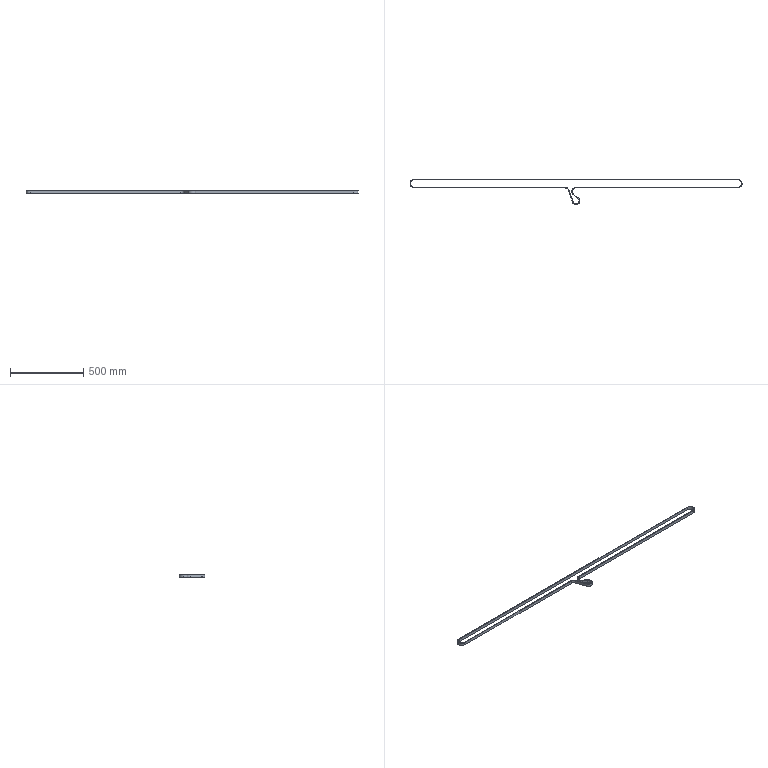Part | STEP file | Guide wheel mechanism revised.sldasm-Part-73 | 1 solid | 26 faces | box 2259 x 173.965 x 20 mm | volume 434312 mm3 | cylinder 14 | plane 12 | commonest cylinder face diameters 50 x6 59 x6 41.93 x1 51.93 x1
STEP:
#1=CARTESIAN_POINT('',(1081.857,-77.761,10.));
#2=VERTEX_POINT('',#1);
#3=CARTESIAN_POINT('',(1070.5,-54.5,10.));
#4=VERTEX_POINT('',#3);
#5=CARTESIAN_POINT('',(1100.,-54.5,10.));
#6=DIRECTION('',(0.,0.,-1.));
#7=DIRECTION('',(-1.,0.,0.));
#8=AXIS2_PLACEMENT_3D('',#5,#6,#7);
#9=CIRCLE('',#8,29.5);
#10=EDGE_CURVE('',#2,#4,#9,.T.);
#11=ORIENTED_EDGE('',*,*,#10,.T.);
#12=CARTESIAN_POINT('',(1070.5,-54.5,-10.));
#13=VERTEX_POINT('',#12);
#14=CARTESIAN_POINT('',(1070.5,-54.5,10.));
#15=DIRECTION('',(0.,0.,-1.));
#16=VECTOR('',#15,1000.);
#17=LINE('',#14,#16);
#18=EDGE_CURVE('',#4,#13,#17,.T.);
#19=ORIENTED_EDGE('',*,*,#18,.T.);
#20=CARTESIAN_POINT('',(1081.857,-77.761,-10.));
#21=VERTEX_POINT('',#20);
#22=CARTESIAN_POINT('',(1100.,-54.5,-10.));
#23=DIRECTION('',(0.,0.,-1.));
#24=DIRECTION('',(-1.,0.,0.));
#25=AXIS2_PLACEMENT_3D('',#22,#23,#24);
#26=CIRCLE('',#25,29.5);
#27=EDGE_CURVE('',#21,#13,#26,.T.);
#28=ORIENTED_EDGE('',*,*,#27,.F.);
#29=CARTESIAN_POINT('',(1081.857,-77.761,10.));
#30=DIRECTION('',(0.,0.,-1.));
#31=VECTOR('',#30,1000.);
#32=LINE('',#29,#31);
#33=EDGE_CURVE('',#2,#21,#32,.T.);
#34=ORIENTED_EDGE('',*,*,#33,.F.);
#35=EDGE_LOOP('',(#11,#19,#28,#34));
#36=FACE_OUTER_BOUND('',#35,.T.);
#37=CARTESIAN_POINT('',(1100.,-54.5,10.));
#38=DIRECTION('',(0.,0.,-1.));
#39=DIRECTION('',(-1.,0.,0.));
#40=AXIS2_PLACEMENT_3D('',#37,#38,#39);
#41=CYLINDRICAL_SURFACE('',#40,29.5);
#42=ADVANCED_FACE('',(#36),#41,.T.);
#43=CARTESIAN_POINT('',(0.,25.,10.));
#44=VERTEX_POINT('',#43);
#45=CARTESIAN_POINT('',(-25.,0.,10.));
#46=VERTEX_POINT('',#45);
#47=CARTESIAN_POINT('',(0.,0.,10.));
#48=DIRECTION('',(0.,0.,1.));
#49=DIRECTION('',(1.,0.,0.));
#50=AXIS2_PLACEMENT_3D('',#47,#48,#49);
#51=CIRCLE('',#50,25.);
#52=EDGE_CURVE('',#44,#46,#51,.T.);
#53=ORIENTED_EDGE('',*,*,#52,.T.);
#54=CARTESIAN_POINT('',(-25.,0.,-10.));
#55=VERTEX_POINT('',#54);
#56=CARTESIAN_POINT('',(-25.,0.,10.));
#57=DIRECTION('',(0.,0.,-1.));
#58=VECTOR('',#57,1000.);
#59=LINE('',#56,#58);
#60=EDGE_CURVE('',#46,#55,#59,.T.);
#61=ORIENTED_EDGE('',*,*,#60,.T.);
#62=CARTESIAN_POINT('',(0.,25.,-10.));
#63=VERTEX_POINT('',#62);
#64=CARTESIAN_POINT('',(0.,0.,-10.));
#65=DIRECTION('',(0.,0.,1.));
#66=DIRECTION('',(1.,0.,0.));
#67=AXIS2_PLACEMENT_3D('',#64,#65,#66);
#68=CIRCLE('',#67,25.);
#69=EDGE_CURVE('',#63,#55,#68,.T.);
#70=ORIENTED_EDGE('',*,*,#69,.F.);
#71=CARTESIAN_POINT('',(0.,25.,10.));
#72=DIRECTION('',(0.,0.,-1.));
#73=VECTOR('',#72,1000.);
#74=LINE('',#71,#73);
#75=EDGE_CURVE('',#44,#63,#74,.T.);
#76=ORIENTED_EDGE('',*,*,#75,.F.);
#77=EDGE_LOOP('',(#53,#61,#70,#76));
#78=FACE_OUTER_BOUND('',#77,.T.);
#79=CARTESIAN_POINT('',(0.,0.,10.));
#80=DIRECTION('',(0.,0.,-1.));
#81=DIRECTION('',(-1.,0.,0.));
#82=AXIS2_PLACEMENT_3D('',#79,#80,#81);
#83=CYLINDRICAL_SURFACE('',#82,25.);
#84=ADVANCED_FACE('',(#78),#83,.F.);
#85=CARTESIAN_POINT('',(1075.,-54.5,10.));
#86=VERTEX_POINT('',#85);
#87=CARTESIAN_POINT('',(1100.,-29.5,10.));
#88=VERTEX_POINT('',#87);
#89=CARTESIAN_POINT('',(1100.,-54.5,10.));
#90=DIRECTION('',(0.,0.,-1.));
#91=DIRECTION('',(-1.,0.,0.));
#92=AXIS2_PLACEMENT_3D('',#89,#90,#91);
#93=CIRCLE('',#92,25.);
#94=EDGE_CURVE('',#86,#88,#93,.T.);
#95=ORIENTED_EDGE('',*,*,#94,.F.);
#96=CARTESIAN_POINT('',(1075.,-54.5,-10.));
#97=VERTEX_POINT('',#96);
#98=CARTESIAN_POINT('',(1075.,-54.5,10.));
#99=DIRECTION('',(0.,0.,-1.));
#100=VECTOR('',#99,1000.);
#101=LINE('',#98,#100);
#102=EDGE_CURVE('',#86,#97,#101,.T.);
#103=ORIENTED_EDGE('',*,*,#102,.T.);
#104=CARTESIAN_POINT('',(1100.,-29.5,-10.));
#105=VERTEX_POINT('',#104);
#106=CARTESIAN_POINT('',(1100.,-54.5,-10.));
#107=DIRECTION('',(0.,0.,-1.));
#108=DIRECTION('',(-1.,0.,0.));
#109=AXIS2_PLACEMENT_3D('',#106,#107,#108);
#110=CIRCLE('',#109,25.);
#111=EDGE_CURVE('',#97,#105,#110,.T.);
#112=ORIENTED_EDGE('',*,*,#111,.T.);
#113=CARTESIAN_POINT('',(1100.,-29.5,10.));
#114=DIRECTION('',(0.,0.,-1.));
#115=VECTOR('',#114,1000.);
#116=LINE('',#113,#115);
#117=EDGE_CURVE('',#88,#105,#116,.T.);
#118=ORIENTED_EDGE('',*,*,#117,.F.);
#119=EDGE_LOOP('',(#95,#103,#112,#118));
#120=FACE_OUTER_BOUND('',#119,.T.);
#121=CARTESIAN_POINT('',(1100.,-54.5,10.));
#122=DIRECTION('',(0.,0.,-1.));
#123=DIRECTION('',(-1.,0.,0.));
#124=AXIS2_PLACEMENT_3D('',#121,#122,#123);
#125=CYLINDRICAL_SURFACE('',#124,25.);
#126=ADVANCED_FACE('',(#120),#125,.F.);
#127=CARTESIAN_POINT('',(-29.5,0.,10.));
#128=VERTEX_POINT('',#127);
#129=CARTESIAN_POINT('',(0.,-29.5,10.));
#130=VERTEX_POINT('',#129);
#131=CARTESIAN_POINT('',(0.,0.,10.));
#132=DIRECTION('',(0.,0.,1.));
#133=DIRECTION('',(1.,0.,0.));
#134=AXIS2_PLACEMENT_3D('',#131,#132,#133);
#135=CIRCLE('',#134,29.5);
#136=EDGE_CURVE('',#128,#130,#135,.T.);
#137=ORIENTED_EDGE('',*,*,#136,.F.);
#138=CARTESIAN_POINT('',(-29.5,0.,-10.));
#139=VERTEX_POINT('',#138);
#140=CARTESIAN_POINT('',(-29.5,0.,10.));
#141=DIRECTION('',(0.,0.,-1.));
#142=VECTOR('',#141,1000.);
#143=LINE('',#140,#142);
#144=EDGE_CURVE('',#128,#139,#143,.T.);
#145=ORIENTED_EDGE('',*,*,#144,.T.);
#146=CARTESIAN_POINT('',(0.,-29.5,-10.));
#147=VERTEX_POINT('',#146);
#148=CARTESIAN_POINT('',(0.,0.,-10.));
#149=DIRECTION('',(0.,0.,1.));
#150=DIRECTION('',(1.,0.,0.));
#151=AXIS2_PLACEMENT_3D('',#148,#149,#150);
#152=CIRCLE('',#151,29.5);
#153=EDGE_CURVE('',#139,#147,#152,.T.);
#154=ORIENTED_EDGE('',*,*,#153,.T.);
#155=CARTESIAN_POINT('',(0.,-29.5,10.));
#156=DIRECTION('',(0.,0.,-1.));
#157=VECTOR('',#156,1000.);
#158=LINE('',#155,#157);
#159=EDGE_CURVE('',#130,#147,#158,.T.);
#160=ORIENTED_EDGE('',*,*,#159,.F.);
#161=EDGE_LOOP('',(#137,#145,#154,#160));
#162=FACE_OUTER_BOUND('',#161,.T.);
#163=CARTESIAN_POINT('',(0.,0.,10.));
#164=DIRECTION('',(0.,0.,-1.));
#165=DIRECTION('',(-1.,0.,0.));
#166=AXIS2_PLACEMENT_3D('',#163,#164,#165);
#167=CYLINDRICAL_SURFACE('',#166,29.5);
#168=ADVANCED_FACE('',(#162),#167,.T.);
#169=CARTESIAN_POINT('',(0.,29.5,10.));
#170=VERTEX_POINT('',#169);
#171=CARTESIAN_POINT('',(0.,0.,10.));
#172=DIRECTION('',(0.,0.,1.));
#173=DIRECTION('',(1.,0.,0.));
#174=AXIS2_PLACEMENT_3D('',#171,#172,#173);
#175=CIRCLE('',#174,29.5);
#176=EDGE_CURVE('',#170,#128,#175,.T.);
#177=ORIENTED_EDGE('',*,*,#176,.T.);
#178=ORIENTED_EDGE('',*,*,#136,.T.);
#179=CARTESIAN_POINT('',(1025.,-29.5,10.));
#180=VERTEX_POINT('',#179);
#181=CARTESIAN_POINT('',(0.,-29.5,10.));
#182=DIRECTION('',(1.,0.,0.));
#183=VECTOR('',#182,1000.);
#184=LINE('',#181,#183);
#185=EDGE_CURVE('',#130,#180,#184,.T.);
#186=ORIENTED_EDGE('',*,*,#185,.T.);
#187=CARTESIAN_POINT('',(1048.722,-46.609,10.));
#188=VERTEX_POINT('',#187);
#189=CARTESIAN_POINT('',(1025.,-54.5,10.));
#190=DIRECTION('',(0.,0.,-1.));
#191=DIRECTION('',(-1.,0.,0.));
#192=AXIS2_PLACEMENT_3D('',#189,#190,#191);
#193=CIRCLE('',#192,25.);
#194=EDGE_CURVE('',#180,#188,#193,.T.);
#195=ORIENTED_EDGE('',*,*,#194,.T.);
#196=CARTESIAN_POINT('',(1075.362,-126.696,10.));
#197=VERTEX_POINT('',#196);
#198=CARTESIAN_POINT('',(1048.722,-46.609,10.));
#199=DIRECTION('',(0.3156,-0.9489,0.));
#200=VECTOR('',#199,1000.);
#201=LINE('',#198,#200);
#202=EDGE_CURVE('',#188,#197,#201,.T.);
#203=ORIENTED_EDGE('',*,*,#202,.T.);
#204=CARTESIAN_POINT('',(1115.705,-97.823,10.));
#205=VERTEX_POINT('',#204);
#206=CARTESIAN_POINT('',(1100.,-118.5,10.));
#207=DIRECTION('',(0.,0.,1.));
#208=DIRECTION('',(1.,0.,0.));
#209=AXIS2_PLACEMENT_3D('',#206,#207,#208);
#210=CIRCLE('',#209,25.965);
#211=EDGE_CURVE('',#197,#205,#210,.T.);
#212=ORIENTED_EDGE('',*,*,#211,.T.);
#213=CARTESIAN_POINT('',(1084.878,-74.408,10.));
#214=VERTEX_POINT('',#213);
#215=CARTESIAN_POINT('',(1115.705,-97.823,10.));
#216=DIRECTION('',(-0.7963,0.6049,0.));
#217=VECTOR('',#216,1000.);
#218=LINE('',#215,#217);
#219=EDGE_CURVE('',#205,#214,#218,.T.);
#220=ORIENTED_EDGE('',*,*,#219,.T.);
#221=CARTESIAN_POINT('',(1100.,-54.5,10.));
#222=DIRECTION('',(0.,0.,-1.));
#223=DIRECTION('',(-1.,0.,0.));
#224=AXIS2_PLACEMENT_3D('',#221,#222,#223);
#225=CIRCLE('',#224,25.);
#226=EDGE_CURVE('',#214,#86,#225,.T.);
#227=ORIENTED_EDGE('',*,*,#226,.T.);
#228=ORIENTED_EDGE('',*,*,#94,.T.);
#229=CARTESIAN_POINT('',(2200.,-29.5,10.));
#230=VERTEX_POINT('',#229);
#231=CARTESIAN_POINT('',(1100.,-29.5,10.));
#232=DIRECTION('',(1.,0.,0.));
#233=VECTOR('',#232,1000.);
#234=LINE('',#231,#233);
#235=EDGE_CURVE('',#88,#230,#234,.T.);
#236=ORIENTED_EDGE('',*,*,#235,.T.);
#237=CARTESIAN_POINT('',(2200.,29.5,10.));
#238=VERTEX_POINT('',#237);
#239=CARTESIAN_POINT('',(2200.,0.,10.));
#240=DIRECTION('',(0.,0.,1.));
#241=DIRECTION('',(1.,0.,0.));
#242=AXIS2_PLACEMENT_3D('',#239,#240,#241);
#243=CIRCLE('',#242,29.5);
#244=EDGE_CURVE('',#230,#238,#243,.T.);
#245=ORIENTED_EDGE('',*,*,#244,.T.);
#246=CARTESIAN_POINT('',(2200.,29.5,10.));
#247=DIRECTION('',(-1.,0.,0.));
#248=VECTOR('',#247,1000.);
#249=LINE('',#246,#248);
#250=EDGE_CURVE('',#238,#170,#249,.T.);
#251=ORIENTED_EDGE('',*,*,#250,.T.);
#252=EDGE_LOOP('',(#177,#178,#186,#195,#203,#212,#220,#227,#228,#236,#245,#251));
#253=FACE_OUTER_BOUND('',#252,.T.);
#254=CARTESIAN_POINT('',(0.,-25.,10.));
#255=VERTEX_POINT('',#254);
#256=CARTESIAN_POINT('',(1025.,-25.,10.));
#257=VERTEX_POINT('',#256);
#258=CARTESIAN_POINT('',(0.,-25.,10.));
#259=DIRECTION('',(1.,0.,0.));
#260=VECTOR('',#259,1000.);
#261=LINE('',#258,#260);
#262=EDGE_CURVE('',#255,#257,#261,.T.);
#263=ORIENTED_EDGE('',*,*,#262,.F.);
#264=CARTESIAN_POINT('',(0.,0.,10.));
#265=DIRECTION('',(0.,0.,1.));
#266=DIRECTION('',(1.,0.,0.));
#267=AXIS2_PLACEMENT_3D('',#264,#265,#266);
#268=CIRCLE('',#267,25.);
#269=EDGE_CURVE('',#46,#255,#268,.T.);
#270=ORIENTED_EDGE('',*,*,#269,.F.);
#271=ORIENTED_EDGE('',*,*,#52,.F.);
#272=CARTESIAN_POINT('',(2200.,25.,10.));
#273=VERTEX_POINT('',#272);
#274=CARTESIAN_POINT('',(2200.,25.,10.));
#275=DIRECTION('',(-1.,0.,0.));
#276=VECTOR('',#275,1000.);
#277=LINE('',#274,#276);
#278=EDGE_CURVE('',#273,#44,#277,.T.);
#279=ORIENTED_EDGE('',*,*,#278,.F.);
#280=CARTESIAN_POINT('',(2200.,-25.,10.));
#281=VERTEX_POINT('',#280);
#282=CARTESIAN_POINT('',(2200.,0.,10.));
#283=DIRECTION('',(0.,0.,1.));
#284=DIRECTION('',(1.,0.,0.));
#285=AXIS2_PLACEMENT_3D('',#282,#283,#284);
#286=CIRCLE('',#285,25.);
#287=EDGE_CURVE('',#281,#273,#286,.T.);
#288=ORIENTED_EDGE('',*,*,#287,.F.);
#289=CARTESIAN_POINT('',(1100.,-25.,10.));
#290=VERTEX_POINT('',#289);
#291=CARTESIAN_POINT('',(1100.,-25.,10.));
#292=DIRECTION('',(1.,0.,0.));
#293=VECTOR('',#292,1000.);
#294=LINE('',#291,#293);
#295=EDGE_CURVE('',#290,#281,#294,.T.);
#296=ORIENTED_EDGE('',*,*,#295,.F.);
#297=CARTESIAN_POINT('',(1100.,-54.5,10.));
#298=DIRECTION('',(0.,0.,-1.));
#299=DIRECTION('',(-1.,0.,0.));
#300=AXIS2_PLACEMENT_3D('',#297,#298,#299);
#301=CIRCLE('',#300,29.5);
#302=EDGE_CURVE('',#4,#290,#301,.T.);
#303=ORIENTED_EDGE('',*,*,#302,.F.);
#304=ORIENTED_EDGE('',*,*,#10,.F.);
#305=CARTESIAN_POINT('',(1112.894,-101.969,10.));
#306=VERTEX_POINT('',#305);
#307=CARTESIAN_POINT('',(1112.894,-101.969,10.));
#308=DIRECTION('',(-0.7885,0.615,0.));
#309=VECTOR('',#308,1000.);
#310=LINE('',#307,#309);
#311=EDGE_CURVE('',#306,#2,#310,.T.);
#312=ORIENTED_EDGE('',*,*,#311,.F.);
#313=CARTESIAN_POINT('',(1080.146,-125.235,10.));
#314=VERTEX_POINT('',#313);
#315=CARTESIAN_POINT('',(1100.,-118.5,10.));
#316=DIRECTION('',(0.,0.,1.));
#317=DIRECTION('',(1.,0.,0.));
#318=AXIS2_PLACEMENT_3D('',#315,#316,#317);
#319=CIRCLE('',#318,20.965);
#320=EDGE_CURVE('',#314,#306,#319,.T.);
#321=ORIENTED_EDGE('',*,*,#320,.F.);
#322=CARTESIAN_POINT('',(1052.936,-45.023,10.));
#323=VERTEX_POINT('',#322);
#324=CARTESIAN_POINT('',(1052.936,-45.023,10.));
#325=DIRECTION('',(0.3212,-0.947,0.));
#326=VECTOR('',#325,1000.);
#327=LINE('',#324,#326);
#328=EDGE_CURVE('',#323,#314,#327,.T.);
#329=ORIENTED_EDGE('',*,*,#328,.F.);
#330=CARTESIAN_POINT('',(1025.,-54.5,10.));
#331=DIRECTION('',(0.,0.,-1.));
#332=DIRECTION('',(-1.,0.,0.));
#333=AXIS2_PLACEMENT_3D('',#330,#331,#332);
#334=CIRCLE('',#333,29.5);
#335=EDGE_CURVE('',#257,#323,#334,.T.);
#336=ORIENTED_EDGE('',*,*,#335,.F.);
#337=EDGE_LOOP('',(#263,#270,#271,#279,#288,#296,#303,#304,#312,#321,#329,#336));
#338=FACE_BOUND('',#337,.T.);
#339=CARTESIAN_POINT('',(0.,0.,10.));
#340=DIRECTION('',(0.,0.,1.));
#341=DIRECTION('',(1.,0.,0.));
#342=AXIS2_PLACEMENT_3D('',#339,#340,#341);
#343=PLANE('',#342);
#344=ADVANCED_FACE('',(#253,#338),#343,.T.);
#345=ORIENTED_EDGE('',*,*,#144,.F.);
#346=ORIENTED_EDGE('',*,*,#176,.F.);
#347=CARTESIAN_POINT('',(0.,29.5,-10.));
#348=VERTEX_POINT('',#347);
#349=CARTESIAN_POINT('',(0.,29.5,10.));
#350=DIRECTION('',(0.,0.,-1.));
#351=VECTOR('',#350,1000.);
#352=LINE('',#349,#351);
#353=EDGE_CURVE('',#170,#348,#352,.T.);
#354=ORIENTED_EDGE('',*,*,#353,.T.);
#355=CARTESIAN_POINT('',(0.,0.,-10.));
#356=DIRECTION('',(0.,0.,1.));
#357=DIRECTION('',(1.,0.,0.));
#358=AXIS2_PLACEMENT_3D('',#355,#356,#357);
#359=CIRCLE('',#358,29.5);
#360=EDGE_CURVE('',#348,#139,#359,.T.);
#361=ORIENTED_EDGE('',*,*,#360,.T.);
#362=EDGE_LOOP('',(#345,#346,#354,#361));
#363=FACE_OUTER_BOUND('',#362,.T.);
#364=CARTESIAN_POINT('',(0.,0.,10.));
#365=DIRECTION('',(0.,0.,-1.));
#366=DIRECTION('',(-1.,0.,0.));
#367=AXIS2_PLACEMENT_3D('',#364,#365,#366);
#368=CYLINDRICAL_SURFACE('',#367,29.5);
#369=ADVANCED_FACE('',(#363),#368,.T.);
#370=ORIENTED_EDGE('',*,*,#159,.T.);
#371=CARTESIAN_POINT('',(1025.,-29.5,-10.));
#372=VERTEX_POINT('',#371);
#373=CARTESIAN_POINT('',(0.,-29.5,-10.));
#374=DIRECTION('',(1.,0.,0.));
#375=VECTOR('',#374,1000.);
#376=LINE('',#373,#375);
#377=EDGE_CURVE('',#147,#372,#376,.T.);
#378=ORIENTED_EDGE('',*,*,#377,.T.);
#379=CARTESIAN_POINT('',(1025.,-29.5,10.));
#380=DIRECTION('',(0.,0.,-1.));
#381=VECTOR('',#380,1000.);
#382=LINE('',#379,#381);
#383=EDGE_CURVE('',#180,#372,#382,.T.);
#384=ORIENTED_EDGE('',*,*,#383,.F.);
#385=ORIENTED_EDGE('',*,*,#185,.F.);
#386=EDGE_LOOP('',(#370,#378,#384,#385));
#387=FACE_OUTER_BOUND('',#386,.T.);
#388=CARTESIAN_POINT('',(0.,-29.5,10.));
#389=DIRECTION('',(0.,1.,0.));
#390=DIRECTION('',(-1.,0.,0.));
#391=AXIS2_PLACEMENT_3D('',#388,#389,#390);
#392=PLANE('',#391);
#393=ADVANCED_FACE('',(#387),#392,.F.);
#394=ORIENTED_EDGE('',*,*,#383,.T.);
#395=CARTESIAN_POINT('',(1048.722,-46.609,-10.));
#396=VERTEX_POINT('',#395);
#397=CARTESIAN_POINT('',(1025.,-54.5,-10.));
#398=DIRECTION('',(0.,0.,-1.));
#399=DIRECTION('',(-1.,0.,0.));
#400=AXIS2_PLACEMENT_3D('',#397,#398,#399);
#401=CIRCLE('',#400,25.);
#402=EDGE_CURVE('',#372,#396,#401,.T.);
#403=ORIENTED_EDGE('',*,*,#402,.T.);
#404=CARTESIAN_POINT('',(1048.722,-46.609,10.));
#405=DIRECTION('',(0.,0.,-1.));
#406=VECTOR('',#405,1000.);
#407=LINE('',#404,#406);
#408=EDGE_CURVE('',#188,#396,#407,.T.);
#409=ORIENTED_EDGE('',*,*,#408,.F.);
#410=ORIENTED_EDGE('',*,*,#194,.F.);
#411=EDGE_LOOP('',(#394,#403,#409,#410));
#412=FACE_OUTER_BOUND('',#411,.T.);
#413=CARTESIAN_POINT('',(1025.,-54.5,10.));
#414=DIRECTION('',(0.,0.,-1.));
#415=DIRECTION('',(-1.,0.,0.));
#416=AXIS2_PLACEMENT_3D('',#413,#414,#415);
#417=CYLINDRICAL_SURFACE('',#416,25.);
#418=ADVANCED_FACE('',(#412),#417,.F.);
#419=ORIENTED_EDGE('',*,*,#408,.T.);
#420=CARTESIAN_POINT('',(1075.362,-126.696,-10.));
#421=VERTEX_POINT('',#420);
#422=CARTESIAN_POINT('',(1048.722,-46.609,-10.));
#423=DIRECTION('',(0.3156,-0.9489,0.));
#424=VECTOR('',#423,1000.);
#425=LINE('',#422,#424);
#426=EDGE_CURVE('',#396,#421,#425,.T.);
#427=ORIENTED_EDGE('',*,*,#426,.T.);
#428=CARTESIAN_POINT('',(1075.362,-126.696,10.));
#429=DIRECTION('',(0.,0.,-1.));
#430=VECTOR('',#429,1000.);
#431=LINE('',#428,#430);
#432=EDGE_CURVE('',#197,#421,#431,.T.);
#433=ORIENTED_EDGE('',*,*,#432,.F.);
#434=ORIENTED_EDGE('',*,*,#202,.F.);
#435=EDGE_LOOP('',(#419,#427,#433,#434));
#436=FACE_OUTER_BOUND('',#435,.T.);
#437=CARTESIAN_POINT('',(1048.722,-46.609,10.));
#438=DIRECTION('',(0.9489,0.3156,0.));
#439=DIRECTION('',(-0.3156,0.9489,0.));
#440=AXIS2_PLACEMENT_3D('',#437,#438,#439);
#441=PLANE('',#440);
#442=ADVANCED_FACE('',(#436),#441,.F.);
#443=ORIENTED_EDGE('',*,*,#432,.T.);
#444=CARTESIAN_POINT('',(1115.705,-97.823,-10.));
#445=VERTEX_POINT('',#444);
#446=CARTESIAN_POINT('',(1100.,-118.5,-10.));
#447=DIRECTION('',(0.,0.,1.));
#448=DIRECTION('',(1.,0.,0.));
#449=AXIS2_PLACEMENT_3D('',#446,#447,#448);
#450=CIRCLE('',#449,25.965);
#451=EDGE_CURVE('',#421,#445,#450,.T.);
#452=ORIENTED_EDGE('',*,*,#451,.T.);
#453=CARTESIAN_POINT('',(1115.705,-97.823,10.));
#454=DIRECTION('',(0.,0.,-1.));
#455=VECTOR('',#454,1000.);
#456=LINE('',#453,#455);
#457=EDGE_CURVE('',#205,#445,#456,.T.);
#458=ORIENTED_EDGE('',*,*,#457,.F.);
#459=ORIENTED_EDGE('',*,*,#211,.F.);
#460=EDGE_LOOP('',(#443,#452,#458,#459));
#461=FACE_OUTER_BOUND('',#460,.T.);
#462=CARTESIAN_POINT('',(1100.,-118.5,10.));
#463=DIRECTION('',(0.,0.,-1.));
#464=DIRECTION('',(-1.,0.,0.));
#465=AXIS2_PLACEMENT_3D('',#462,#463,#464);
#466=CYLINDRICAL_SURFACE('',#465,25.965);
#467=ADVANCED_FACE('',(#461),#466,.T.);
#468=ORIENTED_EDGE('',*,*,#457,.T.);
#469=CARTESIAN_POINT('',(1084.878,-74.408,-10.));
#470=VERTEX_POINT('',#469);
#471=CARTESIAN_POINT('',(1115.705,-97.823,-10.));
#472=DIRECTION('',(-0.7963,0.6049,0.));
#473=VECTOR('',#472,1000.);
#474=LINE('',#471,#473);
#475=EDGE_CURVE('',#445,#470,#474,.T.);
#476=ORIENTED_EDGE('',*,*,#475,.T.);
#477=CARTESIAN_POINT('',(1084.878,-74.408,10.));
#478=DIRECTION('',(0.,0.,-1.));
#479=VECTOR('',#478,1000.);
#480=LINE('',#477,#479);
#481=EDGE_CURVE('',#214,#470,#480,.T.);
#482=ORIENTED_EDGE('',*,*,#481,.F.);
#483=ORIENTED_EDGE('',*,*,#219,.F.);
#484=EDGE_LOOP('',(#468,#476,#482,#483));
#485=FACE_OUTER_BOUND('',#484,.T.);
#486=CARTESIAN_POINT('',(1115.705,-97.823,10.));
#487=DIRECTION('',(-0.6049,-0.7963,0.));
#488=DIRECTION('',(0.7963,-0.6049,0.));
#489=AXIS2_PLACEMENT_3D('',#486,#487,#488);
#490=PLANE('',#489);
#491=ADVANCED_FACE('',(#485),#490,.F.);
#492=ORIENTED_EDGE('',*,*,#102,.F.);
#493=ORIENTED_EDGE('',*,*,#226,.F.);
#494=ORIENTED_EDGE('',*,*,#481,.T.);
#495=CARTESIAN_POINT('',(1100.,-54.5,-10.));
#496=DIRECTION('',(0.,0.,-1.));
#497=DIRECTION('',(-1.,0.,0.));
#498=AXIS2_PLACEMENT_3D('',#495,#496,#497);
#499=CIRCLE('',#498,25.);
#500=EDGE_CURVE('',#470,#97,#499,.T.);
#501=ORIENTED_EDGE('',*,*,#500,.T.);
#502=EDGE_LOOP('',(#492,#493,#494,#501));
#503=FACE_OUTER_BOUND('',#502,.T.);
#504=CARTESIAN_POINT('',(1100.,-54.5,10.));
#505=DIRECTION('',(0.,0.,-1.));
#506=DIRECTION('',(-1.,0.,0.));
#507=AXIS2_PLACEMENT_3D('',#504,#505,#506);
#508=CYLINDRICAL_SURFACE('',#507,25.);
#509=ADVANCED_FACE('',(#503),#508,.F.);
#510=ORIENTED_EDGE('',*,*,#117,.T.);
#511=CARTESIAN_POINT('',(2200.,-29.5,-10.));
#512=VERTEX_POINT('',#511);
#513=CARTESIAN_POINT('',(1100.,-29.5,-10.));
#514=DIRECTION('',(1.,0.,0.));
#515=VECTOR('',#514,1000.);
#516=LINE('',#513,#515);
#517=EDGE_CURVE('',#105,#512,#516,.T.);
#518=ORIENTED_EDGE('',*,*,#517,.T.);
#519=CARTESIAN_POINT('',(2200.,-29.5,10.));
#520=DIRECTION('',(0.,0.,-1.));
#521=VECTOR('',#520,1000.);
#522=LINE('',#519,#521);
#523=EDGE_CURVE('',#230,#512,#522,.T.);
#524=ORIENTED_EDGE('',*,*,#523,.F.);
#525=ORIENTED_EDGE('',*,*,#235,.F.);
#526=EDGE_LOOP('',(#510,#518,#524,#525));
#527=FACE_OUTER_BOUND('',#526,.T.);
#528=CARTESIAN_POINT('',(1100.,-29.5,10.));
#529=DIRECTION('',(0.,1.,0.));
#530=DIRECTION('',(-1.,0.,0.));
#531=AXIS2_PLACEMENT_3D('',#528,#529,#530);
#532=PLANE('',#531);
#533=ADVANCED_FACE('',(#527),#532,.F.);
#534=ORIENTED_EDGE('',*,*,#523,.T.);
#535=CARTESIAN_POINT('',(2200.,29.5,-10.));
#536=VERTEX_POINT('',#535);
#537=CARTESIAN_POINT('',(2200.,0.,-10.));
#538=DIRECTION('',(0.,0.,1.));
#539=DIRECTION('',(1.,0.,0.));
#540=AXIS2_PLACEMENT_3D('',#537,#538,#539);
#541=CIRCLE('',#540,29.5);
#542=EDGE_CURVE('',#512,#536,#541,.T.);
#543=ORIENTED_EDGE('',*,*,#542,.T.);
#544=CARTESIAN_POINT('',(2200.,29.5,10.));
#545=DIRECTION('',(0.,0.,-1.));
#546=VECTOR('',#545,1000.);
#547=LINE('',#544,#546);
#548=EDGE_CURVE('',#238,#536,#547,.T.);
#549=ORIENTED_EDGE('',*,*,#548,.F.);
#550=ORIENTED_EDGE('',*,*,#244,.F.);
#551=EDGE_LOOP('',(#534,#543,#549,#550));
#552=FACE_OUTER_BOUND('',#551,.T.);
#553=CARTESIAN_POINT('',(2200.,0.,10.));
#554=DIRECTION('',(0.,0.,-1.));
#555=DIRECTION('',(-1.,0.,0.));
#556=AXIS2_PLACEMENT_3D('',#553,#554,#555);
#557=CYLINDRICAL_SURFACE('',#556,29.5);
#558=ADVANCED_FACE('',(#552),#557,.T.);
#559=ORIENTED_EDGE('',*,*,#548,.T.);
#560=CARTESIAN_POINT('',(2200.,29.5,-10.));
#561=DIRECTION('',(-1.,0.,0.));
#562=VECTOR('',#561,1000.);
#563=LINE('',#560,#562);
#564=EDGE_CURVE('',#536,#348,#563,.T.);
#565=ORIENTED_EDGE('',*,*,#564,.T.);
#566=ORIENTED_EDGE('',*,*,#353,.F.);
#567=ORIENTED_EDGE('',*,*,#250,.F.);
#568=EDGE_LOOP('',(#559,#565,#566,#567));
#569=FACE_OUTER_BOUND('',#568,.T.);
#570=CARTESIAN_POINT('',(2200.,29.5,10.));
#571=DIRECTION('',(0.,-1.,0.));
#572=DIRECTION('',(0.,0.,-1.));
#573=AXIS2_PLACEMENT_3D('',#570,#571,#572);
#574=PLANE('',#573);
#575=ADVANCED_FACE('',(#569),#574,.F.);
#576=ORIENTED_EDGE('',*,*,#60,.F.);
#577=ORIENTED_EDGE('',*,*,#269,.T.);
#578=CARTESIAN_POINT('',(0.,-25.,-10.));
#579=VERTEX_POINT('',#578);
#580=CARTESIAN_POINT('',(0.,-25.,10.));
#581=DIRECTION('',(0.,0.,-1.));
#582=VECTOR('',#581,1000.);
#583=LINE('',#580,#582);
#584=EDGE_CURVE('',#255,#579,#583,.T.);
#585=ORIENTED_EDGE('',*,*,#584,.T.);
#586=CARTESIAN_POINT('',(0.,0.,-10.));
#587=DIRECTION('',(0.,0.,1.));
#588=DIRECTION('',(1.,0.,0.));
#589=AXIS2_PLACEMENT_3D('',#586,#587,#588);
#590=CIRCLE('',#589,25.);
#591=EDGE_CURVE('',#55,#579,#590,.T.);
#592=ORIENTED_EDGE('',*,*,#591,.F.);
#593=EDGE_LOOP('',(#576,#577,#585,#592));
#594=FACE_OUTER_BOUND('',#593,.T.);
#595=CARTESIAN_POINT('',(0.,0.,10.));
#596=DIRECTION('',(0.,0.,-1.));
#597=DIRECTION('',(-1.,0.,0.));
#598=AXIS2_PLACEMENT_3D('',#595,#596,#597);
#599=CYLINDRICAL_SURFACE('',#598,25.);
#600=ADVANCED_FACE('',(#594),#599,.F.);
#601=CARTESIAN_POINT('',(1025.,-25.,-10.));
#602=VERTEX_POINT('',#601);
#603=CARTESIAN_POINT('',(1025.,-25.,10.));
#604=DIRECTION('',(0.,0.,-1.));
#605=VECTOR('',#604,1000.);
#606=LINE('',#603,#605);
#607=EDGE_CURVE('',#257,#602,#606,.T.);
#608=ORIENTED_EDGE('',*,*,#607,.T.);
#609=CARTESIAN_POINT('',(0.,-25.,-10.));
#610=DIRECTION('',(1.,0.,0.));
#611=VECTOR('',#610,1000.);
#612=LINE('',#609,#611);
#613=EDGE_CURVE('',#579,#602,#612,.T.);
#614=ORIENTED_EDGE('',*,*,#613,.F.);
#615=ORIENTED_EDGE('',*,*,#584,.F.);
#616=ORIENTED_EDGE('',*,*,#262,.T.);
#617=EDGE_LOOP('',(#608,#614,#615,#616));
#618=FACE_OUTER_BOUND('',#617,.T.);
#619=CARTESIAN_POINT('',(0.,-25.,10.));
#620=DIRECTION('',(0.,1.,0.));
#621=DIRECTION('',(-1.,0.,0.));
#622=AXIS2_PLACEMENT_3D('',#619,#620,#621);
#623=PLANE('',#622);
#624=ADVANCED_FACE('',(#618),#623,.T.);
#625=CARTESIAN_POINT('',(1052.936,-45.023,-10.));
#626=VERTEX_POINT('',#625);
#627=CARTESIAN_POINT('',(1052.936,-45.023,10.));
#628=DIRECTION('',(0.,0.,-1.));
#629=VECTOR('',#628,1000.);
#630=LINE('',#627,#629);
#631=EDGE_CURVE('',#323,#626,#630,.T.);
#632=ORIENTED_EDGE('',*,*,#631,.T.);
#633=CARTESIAN_POINT('',(1025.,-54.5,-10.));
#634=DIRECTION('',(0.,0.,-1.));
#635=DIRECTION('',(-1.,0.,0.));
#636=AXIS2_PLACEMENT_3D('',#633,#634,#635);
#637=CIRCLE('',#636,29.5);
#638=EDGE_CURVE('',#602,#626,#637,.T.);
#639=ORIENTED_EDGE('',*,*,#638,.F.);
#640=ORIENTED_EDGE('',*,*,#607,.F.);
#641=ORIENTED_EDGE('',*,*,#335,.T.);
#642=EDGE_LOOP('',(#632,#639,#640,#641));
#643=FACE_OUTER_BOUND('',#642,.T.);
#644=CARTESIAN_POINT('',(1025.,-54.5,10.));
#645=DIRECTION('',(0.,0.,-1.));
#646=DIRECTION('',(-1.,0.,0.));
#647=AXIS2_PLACEMENT_3D('',#644,#645,#646);
#648=CYLINDRICAL_SURFACE('',#647,29.5);
#649=ADVANCED_FACE('',(#643),#648,.T.);
#650=CARTESIAN_POINT('',(1080.146,-125.235,-10.));
#651=VERTEX_POINT('',#650);
#652=CARTESIAN_POINT('',(1080.146,-125.235,10.));
#653=DIRECTION('',(0.,0.,-1.));
#654=VECTOR('',#653,1000.);
#655=LINE('',#652,#654);
#656=EDGE_CURVE('',#314,#651,#655,.T.);
#657=ORIENTED_EDGE('',*,*,#656,.T.);
#658=CARTESIAN_POINT('',(1052.936,-45.023,-10.));
#659=DIRECTION('',(0.3212,-0.947,0.));
#660=VECTOR('',#659,1000.);
#661=LINE('',#658,#660);
#662=EDGE_CURVE('',#626,#651,#661,.T.);
#663=ORIENTED_EDGE('',*,*,#662,.F.);
#664=ORIENTED_EDGE('',*,*,#631,.F.);
#665=ORIENTED_EDGE('',*,*,#328,.T.);
#666=EDGE_LOOP('',(#657,#663,#664,#665));
#667=FACE_OUTER_BOUND('',#666,.T.);
#668=CARTESIAN_POINT('',(1052.936,-45.023,10.));
#669=DIRECTION('',(0.947,0.3212,0.));
#670=DIRECTION('',(-0.3212,0.947,0.));
#671=AXIS2_PLACEMENT_3D('',#668,#669,#670);
#672=PLANE('',#671);
#673=ADVANCED_FACE('',(#667),#672,.T.);
#674=CARTESIAN_POINT('',(1112.894,-101.969,-10.));
#675=VERTEX_POINT('',#674);
#676=CARTESIAN_POINT('',(1112.894,-101.969,10.));
#677=DIRECTION('',(0.,0.,-1.));
#678=VECTOR('',#677,1000.);
#679=LINE('',#676,#678);
#680=EDGE_CURVE('',#306,#675,#679,.T.);
#681=ORIENTED_EDGE('',*,*,#680,.T.);
#682=CARTESIAN_POINT('',(1100.,-118.5,-10.));
#683=DIRECTION('',(0.,0.,1.));
#684=DIRECTION('',(1.,0.,0.));
#685=AXIS2_PLACEMENT_3D('',#682,#683,#684);
#686=CIRCLE('',#685,20.965);
#687=EDGE_CURVE('',#651,#675,#686,.T.);
#688=ORIENTED_EDGE('',*,*,#687,.F.);
#689=ORIENTED_EDGE('',*,*,#656,.F.);
#690=ORIENTED_EDGE('',*,*,#320,.T.);
#691=EDGE_LOOP('',(#681,#688,#689,#690));
#692=FACE_OUTER_BOUND('',#691,.T.);
#693=CARTESIAN_POINT('',(1100.,-118.5,10.));
#694=DIRECTION('',(0.,0.,-1.));
#695=DIRECTION('',(-1.,0.,0.));
#696=AXIS2_PLACEMENT_3D('',#693,#694,#695);
#697=CYLINDRICAL_SURFACE('',#696,20.965);
#698=ADVANCED_FACE('',(#692),#697,.F.);
#699=ORIENTED_EDGE('',*,*,#33,.T.);
#700=CARTESIAN_POINT('',(1112.894,-101.969,-10.));
#701=DIRECTION('',(-0.7885,0.615,0.));
#702=VECTOR('',#701,1000.);
#703=LINE('',#700,#702);
#704=EDGE_CURVE('',#675,#21,#703,.T.);
#705=ORIENTED_EDGE('',*,*,#704,.F.);
#706=ORIENTED_EDGE('',*,*,#680,.F.);
#707=ORIENTED_EDGE('',*,*,#311,.T.);
#708=EDGE_LOOP('',(#699,#705,#706,#707));
#709=FACE_OUTER_BOUND('',#708,.T.);
#710=CARTESIAN_POINT('',(1112.894,-101.969,10.));
#711=DIRECTION('',(-0.615,-0.7885,0.));
#712=DIRECTION('',(0.7885,-0.615,0.));
#713=AXIS2_PLACEMENT_3D('',#710,#711,#712);
#714=PLANE('',#713);
#715=ADVANCED_FACE('',(#709),#714,.T.);
#716=ORIENTED_EDGE('',*,*,#18,.F.);
#717=ORIENTED_EDGE('',*,*,#302,.T.);
#718=CARTESIAN_POINT('',(1100.,-25.,-10.));
#719=VERTEX_POINT('',#718);
#720=CARTESIAN_POINT('',(1100.,-25.,10.));
#721=DIRECTION('',(0.,0.,-1.));
#722=VECTOR('',#721,1000.);
#723=LINE('',#720,#722);
#724=EDGE_CURVE('',#290,#719,#723,.T.);
#725=ORIENTED_EDGE('',*,*,#724,.T.);
#726=CARTESIAN_POINT('',(1100.,-54.5,-10.));
#727=DIRECTION('',(0.,0.,-1.));
#728=DIRECTION('',(-1.,0.,0.));
#729=AXIS2_PLACEMENT_3D('',#726,#727,#728);
#730=CIRCLE('',#729,29.5);
#731=EDGE_CURVE('',#13,#719,#730,.T.);
#732=ORIENTED_EDGE('',*,*,#731,.F.);
#733=EDGE_LOOP('',(#716,#717,#725,#732));
#734=FACE_OUTER_BOUND('',#733,.T.);
#735=CARTESIAN_POINT('',(1100.,-54.5,10.));
#736=DIRECTION('',(0.,0.,-1.));
#737=DIRECTION('',(-1.,0.,0.));
#738=AXIS2_PLACEMENT_3D('',#735,#736,#737);
#739=CYLINDRICAL_SURFACE('',#738,29.5);
#740=ADVANCED_FACE('',(#734),#739,.T.);
#741=CARTESIAN_POINT('',(2200.,-25.,-10.));
#742=VERTEX_POINT('',#741);
#743=CARTESIAN_POINT('',(2200.,-25.,10.));
#744=DIRECTION('',(0.,0.,-1.));
#745=VECTOR('',#744,1000.);
#746=LINE('',#743,#745);
#747=EDGE_CURVE('',#281,#742,#746,.T.);
#748=ORIENTED_EDGE('',*,*,#747,.T.);
#749=CARTESIAN_POINT('',(1100.,-25.,-10.));
#750=DIRECTION('',(1.,0.,0.));
#751=VECTOR('',#750,1000.);
#752=LINE('',#749,#751);
#753=EDGE_CURVE('',#719,#742,#752,.T.);
#754=ORIENTED_EDGE('',*,*,#753,.F.);
#755=ORIENTED_EDGE('',*,*,#724,.F.);
#756=ORIENTED_EDGE('',*,*,#295,.T.);
#757=EDGE_LOOP('',(#748,#754,#755,#756));
#758=FACE_OUTER_BOUND('',#757,.T.);
#759=CARTESIAN_POINT('',(1100.,-25.,10.));
#760=DIRECTION('',(0.,1.,0.));
#761=DIRECTION('',(0.,0.,1.));
#762=AXIS2_PLACEMENT_3D('',#759,#760,#761);
#763=PLANE('',#762);
#764=ADVANCED_FACE('',(#758),#763,.T.);
#765=CARTESIAN_POINT('',(2200.,25.,-10.));
#766=VERTEX_POINT('',#765);
#767=CARTESIAN_POINT('',(2200.,25.,10.));
#768=DIRECTION('',(0.,0.,-1.));
#769=VECTOR('',#768,1000.);
#770=LINE('',#767,#769);
#771=EDGE_CURVE('',#273,#766,#770,.T.);
#772=ORIENTED_EDGE('',*,*,#771,.T.);
#773=CARTESIAN_POINT('',(2200.,0.,-10.));
#774=DIRECTION('',(0.,0.,1.));
#775=DIRECTION('',(1.,0.,0.));
#776=AXIS2_PLACEMENT_3D('',#773,#774,#775);
#777=CIRCLE('',#776,25.);
#778=EDGE_CURVE('',#742,#766,#777,.T.);
#779=ORIENTED_EDGE('',*,*,#778,.F.);
#780=ORIENTED_EDGE('',*,*,#747,.F.);
#781=ORIENTED_EDGE('',*,*,#287,.T.);
#782=EDGE_LOOP('',(#772,#779,#780,#781));
#783=FACE_OUTER_BOUND('',#782,.T.);
#784=CARTESIAN_POINT('',(2200.,0.,10.));
#785=DIRECTION('',(0.,0.,-1.));
#786=DIRECTION('',(-1.,0.,0.));
#787=AXIS2_PLACEMENT_3D('',#784,#785,#786);
#788=CYLINDRICAL_SURFACE('',#787,25.);
#789=ADVANCED_FACE('',(#783),#788,.F.);
#790=ORIENTED_EDGE('',*,*,#75,.T.);
#791=CARTESIAN_POINT('',(2200.,25.,-10.));
#792=DIRECTION('',(-1.,0.,0.));
#793=VECTOR('',#792,1000.);
#794=LINE('',#791,#793);
#795=EDGE_CURVE('',#766,#63,#794,.T.);
#796=ORIENTED_EDGE('',*,*,#795,.F.);
#797=ORIENTED_EDGE('',*,*,#771,.F.);
#798=ORIENTED_EDGE('',*,*,#278,.T.);
#799=EDGE_LOOP('',(#790,#796,#797,#798));
#800=FACE_OUTER_BOUND('',#799,.T.);
#801=CARTESIAN_POINT('',(2200.,25.,10.));
#802=DIRECTION('',(0.,-1.,0.));
#803=DIRECTION('',(0.,0.,-1.));
#804=AXIS2_PLACEMENT_3D('',#801,#802,#803);
#805=PLANE('',#804);
#806=ADVANCED_FACE('',(#800),#805,.T.);
#807=ORIENTED_EDGE('',*,*,#795,.T.);
#808=ORIENTED_EDGE('',*,*,#69,.T.);
#809=ORIENTED_EDGE('',*,*,#591,.T.);
#810=ORIENTED_EDGE('',*,*,#613,.T.);
#811=ORIENTED_EDGE('',*,*,#638,.T.);
#812=ORIENTED_EDGE('',*,*,#662,.T.);
#813=ORIENTED_EDGE('',*,*,#687,.T.);
#814=ORIENTED_EDGE('',*,*,#704,.T.);
#815=ORIENTED_EDGE('',*,*,#27,.T.);
#816=ORIENTED_EDGE('',*,*,#731,.T.);
#817=ORIENTED_EDGE('',*,*,#753,.T.);
#818=ORIENTED_EDGE('',*,*,#778,.T.);
#819=EDGE_LOOP('',(#807,#808,#809,#810,#811,#812,#813,#814,#815,#816,#817,#818));
#820=FACE_BOUND('',#819,.T.);
#821=ORIENTED_EDGE('',*,*,#360,.F.);
#822=ORIENTED_EDGE('',*,*,#564,.F.);
#823=ORIENTED_EDGE('',*,*,#542,.F.);
#824=ORIENTED_EDGE('',*,*,#517,.F.);
#825=ORIENTED_EDGE('',*,*,#111,.F.);
#826=ORIENTED_EDGE('',*,*,#500,.F.);
#827=ORIENTED_EDGE('',*,*,#475,.F.);
#828=ORIENTED_EDGE('',*,*,#451,.F.);
#829=ORIENTED_EDGE('',*,*,#426,.F.);
#830=ORIENTED_EDGE('',*,*,#402,.F.);
#831=ORIENTED_EDGE('',*,*,#377,.F.);
#832=ORIENTED_EDGE('',*,*,#153,.F.);
#833=EDGE_LOOP('',(#821,#822,#823,#824,#825,#826,#827,#828,#829,#830,#831,#832));
#834=FACE_OUTER_BOUND('',#833,.T.);
#835=CARTESIAN_POINT('',(0.,0.,-10.));
#836=DIRECTION('',(0.,0.,1.));
#837=DIRECTION('',(1.,0.,0.));
#838=AXIS2_PLACEMENT_3D('',#835,#836,#837);
#839=PLANE('',#838);
#840=ADVANCED_FACE('',(#820,#834),#839,.F.);
#841=CLOSED_SHELL('',(#42,#84,#126,#168,#344,#369,#393,#418,#442,#467,#491,#509,#533,#558,#575,#600,#624,#649,#673,#698,#715,#740,#764,#789,#806,#840));
#842=MANIFOLD_SOLID_BREP('',#841);
#843=CARTESIAN_POINT('',(0.,0.,0.));
#844=DIRECTION('',(0.,0.,1.));
#845=DIRECTION('',(1.,0.,0.));
#846=AXIS2_PLACEMENT_3D('',#843,#844,#845);
#847=(LENGTH_UNIT()NAMED_UNIT(*)SI_UNIT(.MILLI.,.METRE.));
#848=UNCERTAINTY_MEASURE_WITH_UNIT(LENGTH_MEASURE(0.00001),#847,'','');
#849=(NAMED_UNIT(*)PLANE_ANGLE_UNIT()SI_UNIT($,.RADIAN.));
#850=(NAMED_UNIT(*)SI_UNIT($,.STERADIAN.)SOLID_ANGLE_UNIT());
#851=(GEOMETRIC_REPRESENTATION_CONTEXT(3)GLOBAL_UNCERTAINTY_ASSIGNED_CONTEXT((#848))GLOBAL_UNIT_ASSIGNED_CONTEXT((#847,#849,#850))REPRESENTATION_CONTEXT('',''));
#852=ADVANCED_BREP_SHAPE_REPRESENTATION('',(#842,#846),#851);